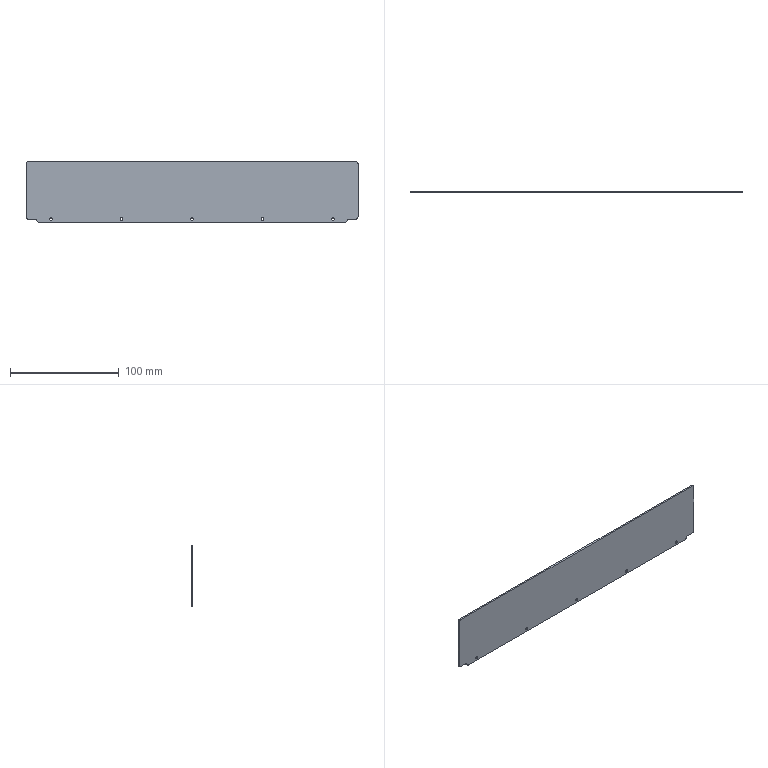Part | NX | features BREP 1 | 1 solid | 36 faces | box 306 x 1.5 x 56 mm | volume 25546 mm3 | cylinder 16 | plane 10 | cone 10 | commonest cylinder face diameters 2.4 x10 4 x6
STEP:
#1=CARTESIAN_POINT('',(-151.,-1.5,28.));
#2=VERTEX_POINT('',#1);
#3=CARTESIAN_POINT('',(-153.,-1.5,26.));
#4=VERTEX_POINT('',#3);
#5=CARTESIAN_POINT('',(-151.,-1.5,26.));
#6=DIRECTION('',(0.,-1.,0.));
#7=DIRECTION('',(0.,0.,1.));
#8=AXIS2_PLACEMENT_3D('',#5,#6,#7);
#9=CIRCLE('',#8,2.);
#10=EDGE_CURVE('',#2,#4,#9,.T.);
#11=ORIENTED_EDGE('',*,*,#10,.F.);
#12=CARTESIAN_POINT('',(-151.,0.,28.));
#13=VERTEX_POINT('',#12);
#14=CARTESIAN_POINT('',(-151.,-1.5,28.));
#15=DIRECTION('',(0.,-1.,0.));
#16=VECTOR('',#15,1000.);
#17=LINE('',#14,#16);
#18=EDGE_CURVE('',#13,#2,#17,.T.);
#19=ORIENTED_EDGE('',*,*,#18,.F.);
#20=CARTESIAN_POINT('',(-153.,0.,26.));
#21=VERTEX_POINT('',#20);
#22=CARTESIAN_POINT('',(-151.,0.,26.));
#23=DIRECTION('',(0.,1.,0.));
#24=DIRECTION('',(0.,0.,1.));
#25=AXIS2_PLACEMENT_3D('',#22,#23,#24);
#26=CIRCLE('',#25,2.);
#27=EDGE_CURVE('',#21,#13,#26,.T.);
#28=ORIENTED_EDGE('',*,*,#27,.F.);
#29=CARTESIAN_POINT('',(-153.,-1.5,26.));
#30=DIRECTION('',(0.,1.,0.));
#31=VECTOR('',#30,1000.);
#32=LINE('',#29,#31);
#33=EDGE_CURVE('',#4,#21,#32,.T.);
#34=ORIENTED_EDGE('',*,*,#33,.F.);
#35=EDGE_LOOP('',(#11,#19,#28,#34));
#36=FACE_BOUND('',#35,.T.);
#37=CARTESIAN_POINT('',(-151.,-1.5,26.));
#38=DIRECTION('',(0.,1.,0.));
#39=DIRECTION('',(0.,0.,1.));
#40=AXIS2_PLACEMENT_3D('',#37,#38,#39);
#41=CYLINDRICAL_SURFACE('',#40,2.);
#42=ADVANCED_FACE('',(#36),#41,.T.);
#43=CARTESIAN_POINT('',(153.,-1.5,26.));
#44=VERTEX_POINT('',#43);
#45=CARTESIAN_POINT('',(151.,-1.5,28.));
#46=VERTEX_POINT('',#45);
#47=CARTESIAN_POINT('',(151.,-1.5,26.));
#48=DIRECTION('',(0.,-1.,0.));
#49=DIRECTION('',(0.,0.,1.));
#50=AXIS2_PLACEMENT_3D('',#47,#48,#49);
#51=CIRCLE('',#50,2.);
#52=EDGE_CURVE('',#44,#46,#51,.T.);
#53=ORIENTED_EDGE('',*,*,#52,.F.);
#54=CARTESIAN_POINT('',(153.,0.,26.));
#55=VERTEX_POINT('',#54);
#56=CARTESIAN_POINT('',(153.,-1.5,26.));
#57=DIRECTION('',(0.,-1.,0.));
#58=VECTOR('',#57,1000.);
#59=LINE('',#56,#58);
#60=EDGE_CURVE('',#55,#44,#59,.T.);
#61=ORIENTED_EDGE('',*,*,#60,.F.);
#62=CARTESIAN_POINT('',(151.,0.,28.));
#63=VERTEX_POINT('',#62);
#64=CARTESIAN_POINT('',(151.,0.,26.));
#65=DIRECTION('',(0.,1.,0.));
#66=DIRECTION('',(0.,0.,1.));
#67=AXIS2_PLACEMENT_3D('',#64,#65,#66);
#68=CIRCLE('',#67,2.);
#69=EDGE_CURVE('',#63,#55,#68,.T.);
#70=ORIENTED_EDGE('',*,*,#69,.F.);
#71=CARTESIAN_POINT('',(151.,-1.5,28.));
#72=DIRECTION('',(0.,1.,0.));
#73=VECTOR('',#72,1000.);
#74=LINE('',#71,#73);
#75=EDGE_CURVE('',#46,#63,#74,.T.);
#76=ORIENTED_EDGE('',*,*,#75,.F.);
#77=EDGE_LOOP('',(#53,#61,#70,#76));
#78=FACE_BOUND('',#77,.T.);
#79=CARTESIAN_POINT('',(151.,-1.5,26.));
#80=DIRECTION('',(0.,1.,0.));
#81=DIRECTION('',(0.,0.,1.));
#82=AXIS2_PLACEMENT_3D('',#79,#80,#81);
#83=CYLINDRICAL_SURFACE('',#82,2.);
#84=ADVANCED_FACE('',(#78),#83,.T.);
#85=CARTESIAN_POINT('',(151.,-1.5,-25.));
#86=VERTEX_POINT('',#85);
#87=CARTESIAN_POINT('',(153.,-1.5,-23.));
#88=VERTEX_POINT('',#87);
#89=CARTESIAN_POINT('',(151.,-1.5,-23.));
#90=DIRECTION('',(0.,-1.,0.));
#91=DIRECTION('',(0.,0.,1.));
#92=AXIS2_PLACEMENT_3D('',#89,#90,#91);
#93=CIRCLE('',#92,2.);
#94=EDGE_CURVE('',#86,#88,#93,.T.);
#95=ORIENTED_EDGE('',*,*,#94,.F.);
#96=CARTESIAN_POINT('',(151.,0.,-25.));
#97=VERTEX_POINT('',#96);
#98=CARTESIAN_POINT('',(151.,-1.5,-25.));
#99=DIRECTION('',(0.,-1.,0.));
#100=VECTOR('',#99,1000.);
#101=LINE('',#98,#100);
#102=EDGE_CURVE('',#97,#86,#101,.T.);
#103=ORIENTED_EDGE('',*,*,#102,.F.);
#104=CARTESIAN_POINT('',(153.,0.,-23.));
#105=VERTEX_POINT('',#104);
#106=CARTESIAN_POINT('',(151.,0.,-23.));
#107=DIRECTION('',(0.,1.,0.));
#108=DIRECTION('',(0.,0.,1.));
#109=AXIS2_PLACEMENT_3D('',#106,#107,#108);
#110=CIRCLE('',#109,2.);
#111=EDGE_CURVE('',#105,#97,#110,.T.);
#112=ORIENTED_EDGE('',*,*,#111,.F.);
#113=CARTESIAN_POINT('',(153.,0.,-23.));
#114=DIRECTION('',(0.,1.,0.));
#115=VECTOR('',#114,1000.);
#116=LINE('',#113,#115);
#117=EDGE_CURVE('',#88,#105,#116,.T.);
#118=ORIENTED_EDGE('',*,*,#117,.F.);
#119=EDGE_LOOP('',(#95,#103,#112,#118));
#120=FACE_BOUND('',#119,.T.);
#121=CARTESIAN_POINT('',(151.,-1.5,-23.));
#122=DIRECTION('',(0.,-1.,0.));
#123=DIRECTION('',(0.,0.,-1.));
#124=AXIS2_PLACEMENT_3D('',#121,#122,#123);
#125=CYLINDRICAL_SURFACE('',#124,2.);
#126=ADVANCED_FACE('',(#120),#125,.T.);
#127=CARTESIAN_POINT('',(-153.,-1.5,-23.));
#128=VERTEX_POINT('',#127);
#129=CARTESIAN_POINT('',(-151.,-1.5,-25.));
#130=VERTEX_POINT('',#129);
#131=CARTESIAN_POINT('',(-151.,-1.5,-23.));
#132=DIRECTION('',(0.,-1.,0.));
#133=DIRECTION('',(0.,0.,1.));
#134=AXIS2_PLACEMENT_3D('',#131,#132,#133);
#135=CIRCLE('',#134,2.);
#136=EDGE_CURVE('',#128,#130,#135,.T.);
#137=ORIENTED_EDGE('',*,*,#136,.F.);
#138=CARTESIAN_POINT('',(-153.,0.,-23.));
#139=VERTEX_POINT('',#138);
#140=CARTESIAN_POINT('',(-153.,-1.5,-23.));
#141=DIRECTION('',(0.,-1.,0.));
#142=VECTOR('',#141,1000.);
#143=LINE('',#140,#142);
#144=EDGE_CURVE('',#139,#128,#143,.T.);
#145=ORIENTED_EDGE('',*,*,#144,.F.);
#146=CARTESIAN_POINT('',(-151.,0.,-25.));
#147=VERTEX_POINT('',#146);
#148=CARTESIAN_POINT('',(-151.,0.,-23.));
#149=DIRECTION('',(0.,1.,0.));
#150=DIRECTION('',(0.,0.,1.));
#151=AXIS2_PLACEMENT_3D('',#148,#149,#150);
#152=CIRCLE('',#151,2.);
#153=EDGE_CURVE('',#147,#139,#152,.T.);
#154=ORIENTED_EDGE('',*,*,#153,.F.);
#155=CARTESIAN_POINT('',(-151.,0.,-25.));
#156=DIRECTION('',(0.,1.,0.));
#157=VECTOR('',#156,1000.);
#158=LINE('',#155,#157);
#159=EDGE_CURVE('',#130,#147,#158,.T.);
#160=ORIENTED_EDGE('',*,*,#159,.F.);
#161=EDGE_LOOP('',(#137,#145,#154,#160));
#162=FACE_BOUND('',#161,.T.);
#163=CARTESIAN_POINT('',(-151.,-1.5,-23.));
#164=DIRECTION('',(0.,-1.,0.));
#165=DIRECTION('',(0.,0.,-1.));
#166=AXIS2_PLACEMENT_3D('',#163,#164,#165);
#167=CYLINDRICAL_SURFACE('',#166,2.);
#168=ADVANCED_FACE('',(#162),#167,.T.);
#169=CARTESIAN_POINT('',(-143.,-1.5,-26.));
#170=VERTEX_POINT('',#169);
#171=CARTESIAN_POINT('',(-141.,-1.5,-28.));
#172=VERTEX_POINT('',#171);
#173=CARTESIAN_POINT('',(-141.,-1.5,-26.));
#174=DIRECTION('',(0.,-1.,0.));
#175=DIRECTION('',(0.,0.,1.));
#176=AXIS2_PLACEMENT_3D('',#173,#174,#175);
#177=CIRCLE('',#176,2.);
#178=EDGE_CURVE('',#170,#172,#177,.T.);
#179=ORIENTED_EDGE('',*,*,#178,.F.);
#180=CARTESIAN_POINT('',(-143.,0.,-26.));
#181=VERTEX_POINT('',#180);
#182=CARTESIAN_POINT('',(-143.,-1.5,-26.));
#183=DIRECTION('',(0.,-1.,0.));
#184=VECTOR('',#183,1000.);
#185=LINE('',#182,#184);
#186=EDGE_CURVE('',#181,#170,#185,.T.);
#187=ORIENTED_EDGE('',*,*,#186,.F.);
#188=CARTESIAN_POINT('',(-141.,0.,-28.));
#189=VERTEX_POINT('',#188);
#190=CARTESIAN_POINT('',(-141.,0.,-26.));
#191=DIRECTION('',(0.,1.,0.));
#192=DIRECTION('',(0.,0.,1.));
#193=AXIS2_PLACEMENT_3D('',#190,#191,#192);
#194=CIRCLE('',#193,2.);
#195=EDGE_CURVE('',#189,#181,#194,.T.);
#196=ORIENTED_EDGE('',*,*,#195,.F.);
#197=CARTESIAN_POINT('',(-141.,0.,-28.));
#198=DIRECTION('',(0.,1.,0.));
#199=VECTOR('',#198,1000.);
#200=LINE('',#197,#199);
#201=EDGE_CURVE('',#172,#189,#200,.T.);
#202=ORIENTED_EDGE('',*,*,#201,.F.);
#203=EDGE_LOOP('',(#179,#187,#196,#202));
#204=FACE_BOUND('',#203,.T.);
#205=CARTESIAN_POINT('',(-141.,-1.5,-26.));
#206=DIRECTION('',(0.,-1.,0.));
#207=DIRECTION('',(0.,0.,-1.));
#208=AXIS2_PLACEMENT_3D('',#205,#206,#207);
#209=CYLINDRICAL_SURFACE('',#208,2.);
#210=ADVANCED_FACE('',(#204),#209,.T.);
#211=CARTESIAN_POINT('',(141.,-1.5,-28.));
#212=VERTEX_POINT('',#211);
#213=CARTESIAN_POINT('',(143.,-1.5,-26.));
#214=VERTEX_POINT('',#213);
#215=CARTESIAN_POINT('',(141.,-1.5,-26.));
#216=DIRECTION('',(0.,-1.,0.));
#217=DIRECTION('',(0.,0.,1.));
#218=AXIS2_PLACEMENT_3D('',#215,#216,#217);
#219=CIRCLE('',#218,2.);
#220=EDGE_CURVE('',#212,#214,#219,.T.);
#221=ORIENTED_EDGE('',*,*,#220,.F.);
#222=CARTESIAN_POINT('',(141.,0.,-28.));
#223=VERTEX_POINT('',#222);
#224=CARTESIAN_POINT('',(141.,-1.5,-28.));
#225=DIRECTION('',(0.,-1.,0.));
#226=VECTOR('',#225,1000.);
#227=LINE('',#224,#226);
#228=EDGE_CURVE('',#223,#212,#227,.T.);
#229=ORIENTED_EDGE('',*,*,#228,.F.);
#230=CARTESIAN_POINT('',(143.,0.,-26.));
#231=VERTEX_POINT('',#230);
#232=CARTESIAN_POINT('',(141.,0.,-26.));
#233=DIRECTION('',(0.,1.,0.));
#234=DIRECTION('',(0.,0.,1.));
#235=AXIS2_PLACEMENT_3D('',#232,#233,#234);
#236=CIRCLE('',#235,2.);
#237=EDGE_CURVE('',#231,#223,#236,.T.);
#238=ORIENTED_EDGE('',*,*,#237,.F.);
#239=CARTESIAN_POINT('',(143.,0.,-26.));
#240=DIRECTION('',(0.,1.,0.));
#241=VECTOR('',#240,1000.);
#242=LINE('',#239,#241);
#243=EDGE_CURVE('',#214,#231,#242,.T.);
#244=ORIENTED_EDGE('',*,*,#243,.F.);
#245=EDGE_LOOP('',(#221,#229,#238,#244));
#246=FACE_BOUND('',#245,.T.);
#247=CARTESIAN_POINT('',(141.,-1.5,-26.));
#248=DIRECTION('',(0.,-1.,0.));
#249=DIRECTION('',(0.,0.,-1.));
#250=AXIS2_PLACEMENT_3D('',#247,#248,#249);
#251=CYLINDRICAL_SURFACE('',#250,2.);
#252=ADVANCED_FACE('',(#246),#251,.T.);
#253=CARTESIAN_POINT('',(-143.,-1.5,-25.));
#254=VERTEX_POINT('',#253);
#255=CARTESIAN_POINT('',(-153.,-1.5,-25.));
#256=DIRECTION('',(1.,0.,0.));
#257=VECTOR('',#256,1000.);
#258=LINE('',#255,#257);
#259=EDGE_CURVE('',#130,#254,#258,.T.);
#260=ORIENTED_EDGE('',*,*,#259,.F.);
#261=ORIENTED_EDGE('',*,*,#159,.T.);
#262=CARTESIAN_POINT('',(-143.,0.,-25.));
#263=VERTEX_POINT('',#262);
#264=CARTESIAN_POINT('',(-153.,0.,-25.));
#265=DIRECTION('',(1.,0.,0.));
#266=VECTOR('',#265,1000.);
#267=LINE('',#264,#266);
#268=EDGE_CURVE('',#147,#263,#267,.T.);
#269=ORIENTED_EDGE('',*,*,#268,.T.);
#270=CARTESIAN_POINT('',(-143.,-1.5,-25.));
#271=DIRECTION('',(0.,1.,0.));
#272=VECTOR('',#271,1000.);
#273=LINE('',#270,#272);
#274=EDGE_CURVE('',#254,#263,#273,.T.);
#275=ORIENTED_EDGE('',*,*,#274,.F.);
#276=EDGE_LOOP('',(#260,#261,#269,#275));
#277=FACE_BOUND('',#276,.T.);
#278=CARTESIAN_POINT('',(-153.,-1.5,-25.));
#279=DIRECTION('',(0.,0.,1.));
#280=DIRECTION('',(1.,0.,0.));
#281=AXIS2_PLACEMENT_3D('',#278,#279,#280);
#282=PLANE('',#281);
#283=ADVANCED_FACE('',(#277),#282,.F.);
#284=CARTESIAN_POINT('',(-143.,0.,-28.));
#285=DIRECTION('',(0.,0.,-1.));
#286=VECTOR('',#285,1000.);
#287=LINE('',#284,#286);
#288=EDGE_CURVE('',#263,#181,#287,.T.);
#289=ORIENTED_EDGE('',*,*,#288,.T.);
#290=ORIENTED_EDGE('',*,*,#186,.T.);
#291=CARTESIAN_POINT('',(-143.,-1.5,-28.));
#292=DIRECTION('',(0.,0.,-1.));
#293=VECTOR('',#292,1000.);
#294=LINE('',#291,#293);
#295=EDGE_CURVE('',#254,#170,#294,.T.);
#296=ORIENTED_EDGE('',*,*,#295,.F.);
#297=ORIENTED_EDGE('',*,*,#274,.T.);
#298=EDGE_LOOP('',(#289,#290,#296,#297));
#299=FACE_BOUND('',#298,.T.);
#300=CARTESIAN_POINT('',(-143.,-1.5,-28.));
#301=DIRECTION('',(1.,0.,0.));
#302=DIRECTION('',(0.,0.,-1.));
#303=AXIS2_PLACEMENT_3D('',#300,#301,#302);
#304=PLANE('',#303);
#305=ADVANCED_FACE('',(#299),#304,.F.);
#306=CARTESIAN_POINT('',(143.,-1.5,-25.));
#307=VERTEX_POINT('',#306);
#308=CARTESIAN_POINT('',(143.,-1.5,-28.));
#309=DIRECTION('',(0.,0.,1.));
#310=VECTOR('',#309,1000.);
#311=LINE('',#308,#310);
#312=EDGE_CURVE('',#214,#307,#311,.T.);
#313=ORIENTED_EDGE('',*,*,#312,.F.);
#314=ORIENTED_EDGE('',*,*,#243,.T.);
#315=CARTESIAN_POINT('',(143.,0.,-25.));
#316=VERTEX_POINT('',#315);
#317=CARTESIAN_POINT('',(143.,0.,-28.));
#318=DIRECTION('',(0.,0.,1.));
#319=VECTOR('',#318,1000.);
#320=LINE('',#317,#319);
#321=EDGE_CURVE('',#231,#316,#320,.T.);
#322=ORIENTED_EDGE('',*,*,#321,.T.);
#323=CARTESIAN_POINT('',(143.,-1.5,-25.));
#324=DIRECTION('',(0.,1.,0.));
#325=VECTOR('',#324,1000.);
#326=LINE('',#323,#325);
#327=EDGE_CURVE('',#307,#316,#326,.T.);
#328=ORIENTED_EDGE('',*,*,#327,.F.);
#329=EDGE_LOOP('',(#313,#314,#322,#328));
#330=FACE_BOUND('',#329,.T.);
#331=CARTESIAN_POINT('',(143.,-1.5,-28.));
#332=DIRECTION('',(-1.,0.,0.));
#333=DIRECTION('',(0.,0.,1.));
#334=AXIS2_PLACEMENT_3D('',#331,#332,#333);
#335=PLANE('',#334);
#336=ADVANCED_FACE('',(#330),#335,.F.);
#337=CARTESIAN_POINT('',(153.,0.,-25.));
#338=DIRECTION('',(1.,0.,0.));
#339=VECTOR('',#338,1000.);
#340=LINE('',#337,#339);
#341=EDGE_CURVE('',#316,#97,#340,.T.);
#342=ORIENTED_EDGE('',*,*,#341,.T.);
#343=ORIENTED_EDGE('',*,*,#102,.T.);
#344=CARTESIAN_POINT('',(153.,-1.5,-25.));
#345=DIRECTION('',(1.,0.,0.));
#346=VECTOR('',#345,1000.);
#347=LINE('',#344,#346);
#348=EDGE_CURVE('',#307,#86,#347,.T.);
#349=ORIENTED_EDGE('',*,*,#348,.F.);
#350=ORIENTED_EDGE('',*,*,#327,.T.);
#351=EDGE_LOOP('',(#342,#343,#349,#350));
#352=FACE_BOUND('',#351,.T.);
#353=CARTESIAN_POINT('',(153.,-1.5,-25.));
#354=DIRECTION('',(0.,0.,1.));
#355=DIRECTION('',(1.,0.,0.));
#356=AXIS2_PLACEMENT_3D('',#353,#354,#355);
#357=PLANE('',#356);
#358=ADVANCED_FACE('',(#352),#357,.F.);
#359=CARTESIAN_POINT('',(-130.,0.,-27.25));
#360=VERTEX_POINT('',#359);
#361=CARTESIAN_POINT('',(-130.,-1.05,-26.2));
#362=VERTEX_POINT('',#361);
#363=CARTESIAN_POINT('',(-130.,0.,-27.25));
#364=DIRECTION('',(0.,0.7071,-0.7071));
#365=VECTOR('',#364,1000.);
#366=LINE('',#363,#365);
#367=EDGE_CURVE('',#360,#362,#366,.F.);
#368=ORIENTED_EDGE('',*,*,#367,.T.);
#369=CARTESIAN_POINT('',(-130.,-1.05,-23.8));
#370=VERTEX_POINT('',#369);
#371=CARTESIAN_POINT('',(-130.,-1.05,-25.));
#372=DIRECTION('',(0.,1.,0.));
#373=DIRECTION('',(0.,0.,1.));
#374=AXIS2_PLACEMENT_3D('',#371,#372,#373);
#375=CIRCLE('',#374,1.2);
#376=EDGE_CURVE('',#370,#362,#375,.T.);
#377=ORIENTED_EDGE('',*,*,#376,.F.);
#378=CARTESIAN_POINT('',(-130.,0.,-22.75));
#379=VERTEX_POINT('',#378);
#380=CARTESIAN_POINT('',(-130.,0.,-22.75));
#381=DIRECTION('',(0.,0.7071,0.7071));
#382=VECTOR('',#381,1000.);
#383=LINE('',#380,#382);
#384=EDGE_CURVE('',#379,#370,#383,.F.);
#385=ORIENTED_EDGE('',*,*,#384,.F.);
#386=CARTESIAN_POINT('',(-130.,0.,-25.));
#387=DIRECTION('',(0.,1.,0.));
#388=DIRECTION('',(0.,0.,1.));
#389=AXIS2_PLACEMENT_3D('',#386,#387,#388);
#390=CIRCLE('',#389,2.25);
#391=EDGE_CURVE('',#379,#360,#390,.T.);
#392=ORIENTED_EDGE('',*,*,#391,.T.);
#393=EDGE_LOOP('',(#368,#377,#385,#392));
#394=FACE_BOUND('',#393,.T.);
#395=CARTESIAN_POINT('',(-130.,0.,-25.));
#396=DIRECTION('',(0.,1.,0.));
#397=DIRECTION('',(0.,0.,1.));
#398=AXIS2_PLACEMENT_3D('',#395,#396,#397);
#399=CONICAL_SURFACE('',#398,2.25,0.7854);
#400=ADVANCED_FACE('',(#394),#399,.F.);
#401=CARTESIAN_POINT('',(-130.,-1.5,-26.2));
#402=VERTEX_POINT('',#401);
#403=CARTESIAN_POINT('',(-130.,0.,-26.2));
#404=DIRECTION('',(0.,1.,0.));
#405=VECTOR('',#404,1000.);
#406=LINE('',#403,#405);
#407=EDGE_CURVE('',#362,#402,#406,.F.);
#408=ORIENTED_EDGE('',*,*,#407,.T.);
#409=CARTESIAN_POINT('',(-130.,-1.5,-23.8));
#410=VERTEX_POINT('',#409);
#411=CARTESIAN_POINT('',(-130.,-1.5,-25.));
#412=DIRECTION('',(0.,1.,0.));
#413=DIRECTION('',(0.,0.,1.));
#414=AXIS2_PLACEMENT_3D('',#411,#412,#413);
#415=CIRCLE('',#414,1.2);
#416=EDGE_CURVE('',#410,#402,#415,.T.);
#417=ORIENTED_EDGE('',*,*,#416,.F.);
#418=CARTESIAN_POINT('',(-130.,0.,-23.8));
#419=DIRECTION('',(0.,1.,0.));
#420=VECTOR('',#419,1000.);
#421=LINE('',#418,#420);
#422=EDGE_CURVE('',#370,#410,#421,.F.);
#423=ORIENTED_EDGE('',*,*,#422,.F.);
#424=ORIENTED_EDGE('',*,*,#376,.T.);
#425=EDGE_LOOP('',(#408,#417,#423,#424));
#426=FACE_BOUND('',#425,.T.);
#427=CARTESIAN_POINT('',(-130.,0.,-25.));
#428=DIRECTION('',(0.,1.,0.));
#429=DIRECTION('',(0.,0.,1.));
#430=AXIS2_PLACEMENT_3D('',#427,#428,#429);
#431=CYLINDRICAL_SURFACE('',#430,1.2);
#432=ADVANCED_FACE('',(#426),#431,.F.);
#433=CARTESIAN_POINT('',(-65.,0.,-27.25));
#434=VERTEX_POINT('',#433);
#435=CARTESIAN_POINT('',(-65.,-1.05,-26.2));
#436=VERTEX_POINT('',#435);
#437=CARTESIAN_POINT('',(-65.,0.,-27.25));
#438=DIRECTION('',(0.,0.7071,-0.7071));
#439=VECTOR('',#438,1000.);
#440=LINE('',#437,#439);
#441=EDGE_CURVE('',#434,#436,#440,.F.);
#442=ORIENTED_EDGE('',*,*,#441,.T.);
#443=CARTESIAN_POINT('',(-65.,-1.05,-23.8));
#444=VERTEX_POINT('',#443);
#445=CARTESIAN_POINT('',(-65.,-1.05,-25.));
#446=DIRECTION('',(0.,1.,0.));
#447=DIRECTION('',(0.,0.,1.));
#448=AXIS2_PLACEMENT_3D('',#445,#446,#447);
#449=CIRCLE('',#448,1.2);
#450=EDGE_CURVE('',#444,#436,#449,.T.);
#451=ORIENTED_EDGE('',*,*,#450,.F.);
#452=CARTESIAN_POINT('',(-65.,0.,-22.75));
#453=VERTEX_POINT('',#452);
#454=CARTESIAN_POINT('',(-65.,0.,-22.75));
#455=DIRECTION('',(0.,0.7071,0.7071));
#456=VECTOR('',#455,1000.);
#457=LINE('',#454,#456);
#458=EDGE_CURVE('',#453,#444,#457,.F.);
#459=ORIENTED_EDGE('',*,*,#458,.F.);
#460=CARTESIAN_POINT('',(-65.,0.,-25.));
#461=DIRECTION('',(0.,1.,0.));
#462=DIRECTION('',(0.,0.,1.));
#463=AXIS2_PLACEMENT_3D('',#460,#461,#462);
#464=CIRCLE('',#463,2.25);
#465=EDGE_CURVE('',#453,#434,#464,.T.);
#466=ORIENTED_EDGE('',*,*,#465,.T.);
#467=EDGE_LOOP('',(#442,#451,#459,#466));
#468=FACE_BOUND('',#467,.T.);
#469=CARTESIAN_POINT('',(-65.,0.,-25.));
#470=DIRECTION('',(0.,1.,0.));
#471=DIRECTION('',(0.,0.,1.));
#472=AXIS2_PLACEMENT_3D('',#469,#470,#471);
#473=CONICAL_SURFACE('',#472,2.25,0.7854);
#474=ADVANCED_FACE('',(#468),#473,.F.);
#475=CARTESIAN_POINT('',(-65.,-1.5,-26.2));
#476=VERTEX_POINT('',#475);
#477=CARTESIAN_POINT('',(-65.,0.,-26.2));
#478=DIRECTION('',(0.,1.,0.));
#479=VECTOR('',#478,1000.);
#480=LINE('',#477,#479);
#481=EDGE_CURVE('',#436,#476,#480,.F.);
#482=ORIENTED_EDGE('',*,*,#481,.T.);
#483=CARTESIAN_POINT('',(-65.,-1.5,-23.8));
#484=VERTEX_POINT('',#483);
#485=CARTESIAN_POINT('',(-65.,-1.5,-25.));
#486=DIRECTION('',(0.,1.,0.));
#487=DIRECTION('',(0.,0.,1.));
#488=AXIS2_PLACEMENT_3D('',#485,#486,#487);
#489=CIRCLE('',#488,1.2);
#490=EDGE_CURVE('',#484,#476,#489,.T.);
#491=ORIENTED_EDGE('',*,*,#490,.F.);
#492=CARTESIAN_POINT('',(-65.,0.,-23.8));
#493=DIRECTION('',(0.,1.,0.));
#494=VECTOR('',#493,1000.);
#495=LINE('',#492,#494);
#496=EDGE_CURVE('',#444,#484,#495,.F.);
#497=ORIENTED_EDGE('',*,*,#496,.F.);
#498=ORIENTED_EDGE('',*,*,#450,.T.);
#499=EDGE_LOOP('',(#482,#491,#497,#498));
#500=FACE_BOUND('',#499,.T.);
#501=CARTESIAN_POINT('',(-65.,0.,-25.));
#502=DIRECTION('',(0.,1.,0.));
#503=DIRECTION('',(0.,0.,1.));
#504=AXIS2_PLACEMENT_3D('',#501,#502,#503);
#505=CYLINDRICAL_SURFACE('',#504,1.2);
#506=ADVANCED_FACE('',(#500),#505,.F.);
#507=CARTESIAN_POINT('',(0.,0.,-27.25));
#508=VERTEX_POINT('',#507);
#509=CARTESIAN_POINT('',(0.,-1.05,-26.2));
#510=VERTEX_POINT('',#509);
#511=CARTESIAN_POINT('',(0.,0.,-27.25));
#512=DIRECTION('',(0.,0.7071,-0.7071));
#513=VECTOR('',#512,1000.);
#514=LINE('',#511,#513);
#515=EDGE_CURVE('',#508,#510,#514,.F.);
#516=ORIENTED_EDGE('',*,*,#515,.T.);
#517=CARTESIAN_POINT('',(0.,-1.05,-23.8));
#518=VERTEX_POINT('',#517);
#519=CARTESIAN_POINT('',(0.,-1.05,-25.));
#520=DIRECTION('',(0.,1.,0.));
#521=DIRECTION('',(0.,0.,1.));
#522=AXIS2_PLACEMENT_3D('',#519,#520,#521);
#523=CIRCLE('',#522,1.2);
#524=EDGE_CURVE('',#518,#510,#523,.T.);
#525=ORIENTED_EDGE('',*,*,#524,.F.);
#526=CARTESIAN_POINT('',(0.,0.,-22.75));
#527=VERTEX_POINT('',#526);
#528=CARTESIAN_POINT('',(0.,0.,-22.75));
#529=DIRECTION('',(0.,0.7071,0.7071));
#530=VECTOR('',#529,1000.);
#531=LINE('',#528,#530);
#532=EDGE_CURVE('',#527,#518,#531,.F.);
#533=ORIENTED_EDGE('',*,*,#532,.F.);
#534=CARTESIAN_POINT('',(0.,0.,-25.));
#535=DIRECTION('',(0.,1.,0.));
#536=DIRECTION('',(0.,0.,1.));
#537=AXIS2_PLACEMENT_3D('',#534,#535,#536);
#538=CIRCLE('',#537,2.25);
#539=EDGE_CURVE('',#527,#508,#538,.T.);
#540=ORIENTED_EDGE('',*,*,#539,.T.);
#541=EDGE_LOOP('',(#516,#525,#533,#540));
#542=FACE_BOUND('',#541,.T.);
#543=CARTESIAN_POINT('',(0.,0.,-25.));
#544=DIRECTION('',(0.,1.,0.));
#545=DIRECTION('',(0.,0.,1.));
#546=AXIS2_PLACEMENT_3D('',#543,#544,#545);
#547=CONICAL_SURFACE('',#546,2.25,0.7854);
#548=ADVANCED_FACE('',(#542),#547,.F.);
#549=CARTESIAN_POINT('',(0.,-1.5,-26.2));
#550=VERTEX_POINT('',#549);
#551=CARTESIAN_POINT('',(0.,0.,-26.2));
#552=DIRECTION('',(0.,1.,0.));
#553=VECTOR('',#552,1000.);
#554=LINE('',#551,#553);
#555=EDGE_CURVE('',#510,#550,#554,.F.);
#556=ORIENTED_EDGE('',*,*,#555,.T.);
#557=CARTESIAN_POINT('',(0.,-1.5,-23.8));
#558=VERTEX_POINT('',#557);
#559=CARTESIAN_POINT('',(0.,-1.5,-25.));
#560=DIRECTION('',(0.,1.,0.));
#561=DIRECTION('',(0.,0.,1.));
#562=AXIS2_PLACEMENT_3D('',#559,#560,#561);
#563=CIRCLE('',#562,1.2);
#564=EDGE_CURVE('',#558,#550,#563,.T.);
#565=ORIENTED_EDGE('',*,*,#564,.F.);
#566=CARTESIAN_POINT('',(0.,0.,-23.8));
#567=DIRECTION('',(0.,1.,0.));
#568=VECTOR('',#567,1000.);
#569=LINE('',#566,#568);
#570=EDGE_CURVE('',#518,#558,#569,.F.);
#571=ORIENTED_EDGE('',*,*,#570,.F.);
#572=ORIENTED_EDGE('',*,*,#524,.T.);
#573=EDGE_LOOP('',(#556,#565,#571,#572));
#574=FACE_BOUND('',#573,.T.);
#575=CARTESIAN_POINT('',(0.,0.,-25.));
#576=DIRECTION('',(0.,1.,0.));
#577=DIRECTION('',(0.,0.,1.));
#578=AXIS2_PLACEMENT_3D('',#575,#576,#577);
#579=CYLINDRICAL_SURFACE('',#578,1.2);
#580=ADVANCED_FACE('',(#574),#579,.F.);
#581=CARTESIAN_POINT('',(65.,0.,-27.25));
#582=VERTEX_POINT('',#581);
#583=CARTESIAN_POINT('',(65.,-1.05,-26.2));
#584=VERTEX_POINT('',#583);
#585=CARTESIAN_POINT('',(65.,0.,-27.25));
#586=DIRECTION('',(0.,0.7071,-0.7071));
#587=VECTOR('',#586,1000.);
#588=LINE('',#585,#587);
#589=EDGE_CURVE('',#582,#584,#588,.F.);
#590=ORIENTED_EDGE('',*,*,#589,.T.);
#591=CARTESIAN_POINT('',(65.,-1.05,-23.8));
#592=VERTEX_POINT('',#591);
#593=CARTESIAN_POINT('',(65.,-1.05,-25.));
#594=DIRECTION('',(0.,1.,0.));
#595=DIRECTION('',(0.,0.,1.));
#596=AXIS2_PLACEMENT_3D('',#593,#594,#595);
#597=CIRCLE('',#596,1.2);
#598=EDGE_CURVE('',#592,#584,#597,.T.);
#599=ORIENTED_EDGE('',*,*,#598,.F.);
#600=CARTESIAN_POINT('',(65.,0.,-22.75));
#601=VERTEX_POINT('',#600);
#602=CARTESIAN_POINT('',(65.,0.,-22.75));
#603=DIRECTION('',(0.,0.7071,0.7071));
#604=VECTOR('',#603,1000.);
#605=LINE('',#602,#604);
#606=EDGE_CURVE('',#601,#592,#605,.F.);
#607=ORIENTED_EDGE('',*,*,#606,.F.);
#608=CARTESIAN_POINT('',(65.,0.,-25.));
#609=DIRECTION('',(0.,1.,0.));
#610=DIRECTION('',(0.,0.,1.));
#611=AXIS2_PLACEMENT_3D('',#608,#609,#610);
#612=CIRCLE('',#611,2.25);
#613=EDGE_CURVE('',#601,#582,#612,.T.);
#614=ORIENTED_EDGE('',*,*,#613,.T.);
#615=EDGE_LOOP('',(#590,#599,#607,#614));
#616=FACE_BOUND('',#615,.T.);
#617=CARTESIAN_POINT('',(65.,0.,-25.));
#618=DIRECTION('',(0.,1.,0.));
#619=DIRECTION('',(0.,0.,1.));
#620=AXIS2_PLACEMENT_3D('',#617,#618,#619);
#621=CONICAL_SURFACE('',#620,2.25,0.7854);
#622=ADVANCED_FACE('',(#616),#621,.F.);
#623=CARTESIAN_POINT('',(65.,-1.5,-26.2));
#624=VERTEX_POINT('',#623);
#625=CARTESIAN_POINT('',(65.,0.,-26.2));
#626=DIRECTION('',(0.,1.,0.));
#627=VECTOR('',#626,1000.);
#628=LINE('',#625,#627);
#629=EDGE_CURVE('',#584,#624,#628,.F.);
#630=ORIENTED_EDGE('',*,*,#629,.T.);
#631=CARTESIAN_POINT('',(65.,-1.5,-23.8));
#632=VERTEX_POINT('',#631);
#633=CARTESIAN_POINT('',(65.,-1.5,-25.));
#634=DIRECTION('',(0.,1.,0.));
#635=DIRECTION('',(0.,0.,1.));
#636=AXIS2_PLACEMENT_3D('',#633,#634,#635);
#637=CIRCLE('',#636,1.2);
#638=EDGE_CURVE('',#632,#624,#637,.T.);
#639=ORIENTED_EDGE('',*,*,#638,.F.);
#640=CARTESIAN_POINT('',(65.,0.,-23.8));
#641=DIRECTION('',(0.,1.,0.));
#642=VECTOR('',#641,1000.);
#643=LINE('',#640,#642);
#644=EDGE_CURVE('',#592,#632,#643,.F.);
#645=ORIENTED_EDGE('',*,*,#644,.F.);
#646=ORIENTED_EDGE('',*,*,#598,.T.);
#647=EDGE_LOOP('',(#630,#639,#645,#646));
#648=FACE_BOUND('',#647,.T.);
#649=CARTESIAN_POINT('',(65.,0.,-25.));
#650=DIRECTION('',(0.,1.,0.));
#651=DIRECTION('',(0.,0.,1.));
#652=AXIS2_PLACEMENT_3D('',#649,#650,#651);
#653=CYLINDRICAL_SURFACE('',#652,1.2);
#654=ADVANCED_FACE('',(#648),#653,.F.);
#655=CARTESIAN_POINT('',(130.,0.,-27.25));
#656=VERTEX_POINT('',#655);
#657=CARTESIAN_POINT('',(130.,-1.05,-26.2));
#658=VERTEX_POINT('',#657);
#659=CARTESIAN_POINT('',(130.,0.,-27.25));
#660=DIRECTION('',(0.,0.7071,-0.7071));
#661=VECTOR('',#660,1000.);
#662=LINE('',#659,#661);
#663=EDGE_CURVE('',#656,#658,#662,.F.);
#664=ORIENTED_EDGE('',*,*,#663,.T.);
#665=CARTESIAN_POINT('',(130.,-1.05,-23.8));
#666=VERTEX_POINT('',#665);
#667=CARTESIAN_POINT('',(130.,-1.05,-25.));
#668=DIRECTION('',(0.,1.,0.));
#669=DIRECTION('',(0.,0.,1.));
#670=AXIS2_PLACEMENT_3D('',#667,#668,#669);
#671=CIRCLE('',#670,1.2);
#672=EDGE_CURVE('',#666,#658,#671,.T.);
#673=ORIENTED_EDGE('',*,*,#672,.F.);
#674=CARTESIAN_POINT('',(130.,0.,-22.75));
#675=VERTEX_POINT('',#674);
#676=CARTESIAN_POINT('',(130.,0.,-22.75));
#677=DIRECTION('',(0.,0.7071,0.7071));
#678=VECTOR('',#677,1000.);
#679=LINE('',#676,#678);
#680=EDGE_CURVE('',#675,#666,#679,.F.);
#681=ORIENTED_EDGE('',*,*,#680,.F.);
#682=CARTESIAN_POINT('',(130.,0.,-25.));
#683=DIRECTION('',(0.,1.,0.));
#684=DIRECTION('',(0.,0.,1.));
#685=AXIS2_PLACEMENT_3D('',#682,#683,#684);
#686=CIRCLE('',#685,2.25);
#687=EDGE_CURVE('',#675,#656,#686,.T.);
#688=ORIENTED_EDGE('',*,*,#687,.T.);
#689=EDGE_LOOP('',(#664,#673,#681,#688));
#690=FACE_BOUND('',#689,.T.);
#691=CARTESIAN_POINT('',(130.,0.,-25.));
#692=DIRECTION('',(0.,1.,0.));
#693=DIRECTION('',(0.,0.,1.));
#694=AXIS2_PLACEMENT_3D('',#691,#692,#693);
#695=CONICAL_SURFACE('',#694,2.25,0.7854);
#696=ADVANCED_FACE('',(#690),#695,.F.);
#697=CARTESIAN_POINT('',(130.,-1.5,-26.2));
#698=VERTEX_POINT('',#697);
#699=CARTESIAN_POINT('',(130.,0.,-26.2));
#700=DIRECTION('',(0.,1.,0.));
#701=VECTOR('',#700,1000.);
#702=LINE('',#699,#701);
#703=EDGE_CURVE('',#658,#698,#702,.F.);
#704=ORIENTED_EDGE('',*,*,#703,.T.);
#705=CARTESIAN_POINT('',(130.,-1.5,-23.8));
#706=VERTEX_POINT('',#705);
#707=CARTESIAN_POINT('',(130.,-1.5,-25.));
#708=DIRECTION('',(0.,1.,0.));
#709=DIRECTION('',(0.,0.,1.));
#710=AXIS2_PLACEMENT_3D('',#707,#708,#709);
#711=CIRCLE('',#710,1.2);
#712=EDGE_CURVE('',#706,#698,#711,.T.);
#713=ORIENTED_EDGE('',*,*,#712,.F.);
#714=CARTESIAN_POINT('',(130.,0.,-23.8));
#715=DIRECTION('',(0.,1.,0.));
#716=VECTOR('',#715,1000.);
#717=LINE('',#714,#716);
#718=EDGE_CURVE('',#666,#706,#717,.F.);
#719=ORIENTED_EDGE('',*,*,#718,.F.);
#720=ORIENTED_EDGE('',*,*,#672,.T.);
#721=EDGE_LOOP('',(#704,#713,#719,#720));
#722=FACE_BOUND('',#721,.T.);
#723=CARTESIAN_POINT('',(130.,0.,-25.));
#724=DIRECTION('',(0.,1.,0.));
#725=DIRECTION('',(0.,0.,1.));
#726=AXIS2_PLACEMENT_3D('',#723,#724,#725);
#727=CYLINDRICAL_SURFACE('',#726,1.2);
#728=ADVANCED_FACE('',(#722),#727,.F.);
#729=ORIENTED_EDGE('',*,*,#687,.F.);
#730=CARTESIAN_POINT('',(130.,0.,-25.));
#731=DIRECTION('',(0.,1.,0.));
#732=DIRECTION('',(0.,0.,1.));
#733=AXIS2_PLACEMENT_3D('',#730,#731,#732);
#734=CIRCLE('',#733,2.25);
#735=EDGE_CURVE('',#656,#675,#734,.T.);
#736=ORIENTED_EDGE('',*,*,#735,.F.);
#737=EDGE_LOOP('',(#729,#736));
#738=FACE_BOUND('',#737,.T.);
#739=ORIENTED_EDGE('',*,*,#613,.F.);
#740=CARTESIAN_POINT('',(65.,0.,-25.));
#741=DIRECTION('',(0.,1.,0.));
#742=DIRECTION('',(0.,0.,1.));
#743=AXIS2_PLACEMENT_3D('',#740,#741,#742);
#744=CIRCLE('',#743,2.25);
#745=EDGE_CURVE('',#582,#601,#744,.T.);
#746=ORIENTED_EDGE('',*,*,#745,.F.);
#747=EDGE_LOOP('',(#739,#746));
#748=FACE_BOUND('',#747,.T.);
#749=ORIENTED_EDGE('',*,*,#539,.F.);
#750=CARTESIAN_POINT('',(0.,0.,-25.));
#751=DIRECTION('',(0.,1.,0.));
#752=DIRECTION('',(0.,0.,1.));
#753=AXIS2_PLACEMENT_3D('',#750,#751,#752);
#754=CIRCLE('',#753,2.25);
#755=EDGE_CURVE('',#508,#527,#754,.T.);
#756=ORIENTED_EDGE('',*,*,#755,.F.);
#757=EDGE_LOOP('',(#749,#756));
#758=FACE_BOUND('',#757,.T.);
#759=ORIENTED_EDGE('',*,*,#465,.F.);
#760=CARTESIAN_POINT('',(-65.,0.,-25.));
#761=DIRECTION('',(0.,1.,0.));
#762=DIRECTION('',(0.,0.,1.));
#763=AXIS2_PLACEMENT_3D('',#760,#761,#762);
#764=CIRCLE('',#763,2.25);
#765=EDGE_CURVE('',#434,#453,#764,.T.);
#766=ORIENTED_EDGE('',*,*,#765,.F.);
#767=EDGE_LOOP('',(#759,#766));
#768=FACE_BOUND('',#767,.T.);
#769=ORIENTED_EDGE('',*,*,#391,.F.);
#770=CARTESIAN_POINT('',(-130.,0.,-25.));
#771=DIRECTION('',(0.,1.,0.));
#772=DIRECTION('',(0.,0.,1.));
#773=AXIS2_PLACEMENT_3D('',#770,#771,#772);
#774=CIRCLE('',#773,2.25);
#775=EDGE_CURVE('',#360,#379,#774,.T.);
#776=ORIENTED_EDGE('',*,*,#775,.F.);
#777=EDGE_LOOP('',(#769,#776));
#778=FACE_BOUND('',#777,.T.);
#779=ORIENTED_EDGE('',*,*,#321,.F.);
#780=ORIENTED_EDGE('',*,*,#237,.T.);
#781=CARTESIAN_POINT('',(-153.,0.,-28.));
#782=DIRECTION('',(-1.,0.,0.));
#783=VECTOR('',#782,1000.);
#784=LINE('',#781,#783);
#785=EDGE_CURVE('',#223,#189,#784,.T.);
#786=ORIENTED_EDGE('',*,*,#785,.T.);
#787=ORIENTED_EDGE('',*,*,#195,.T.);
#788=ORIENTED_EDGE('',*,*,#288,.F.);
#789=ORIENTED_EDGE('',*,*,#268,.F.);
#790=ORIENTED_EDGE('',*,*,#153,.T.);
#791=CARTESIAN_POINT('',(-153.,0.,-28.));
#792=DIRECTION('',(0.,0.,1.));
#793=VECTOR('',#792,1000.);
#794=LINE('',#791,#793);
#795=EDGE_CURVE('',#139,#21,#794,.T.);
#796=ORIENTED_EDGE('',*,*,#795,.T.);
#797=ORIENTED_EDGE('',*,*,#27,.T.);
#798=CARTESIAN_POINT('',(-153.,0.,28.));
#799=DIRECTION('',(1.,0.,0.));
#800=VECTOR('',#799,1000.);
#801=LINE('',#798,#800);
#802=EDGE_CURVE('',#13,#63,#801,.T.);
#803=ORIENTED_EDGE('',*,*,#802,.T.);
#804=ORIENTED_EDGE('',*,*,#69,.T.);
#805=CARTESIAN_POINT('',(153.,0.,-28.));
#806=DIRECTION('',(0.,0.,-1.));
#807=VECTOR('',#806,1000.);
#808=LINE('',#805,#807);
#809=EDGE_CURVE('',#55,#105,#808,.T.);
#810=ORIENTED_EDGE('',*,*,#809,.T.);
#811=ORIENTED_EDGE('',*,*,#111,.T.);
#812=ORIENTED_EDGE('',*,*,#341,.F.);
#813=EDGE_LOOP('',(#779,#780,#786,#787,#788,#789,#790,#796,#797,#803,#804,#810,#811,#812));
#814=FACE_BOUND('',#813,.T.);
#815=CARTESIAN_POINT('',(0.,0.,0.));
#816=DIRECTION('',(0.,1.,0.));
#817=DIRECTION('',(0.,0.,1.));
#818=AXIS2_PLACEMENT_3D('',#815,#816,#817);
#819=PLANE('',#818);
#820=ADVANCED_FACE('',(#738,#748,#758,#768,#778,#814),#819,.T.);
#821=CARTESIAN_POINT('',(-153.,-1.5,-28.));
#822=DIRECTION('',(-1.,0.,0.));
#823=VECTOR('',#822,1000.);
#824=LINE('',#821,#823);
#825=EDGE_CURVE('',#212,#172,#824,.T.);
#826=ORIENTED_EDGE('',*,*,#825,.F.);
#827=ORIENTED_EDGE('',*,*,#220,.T.);
#828=ORIENTED_EDGE('',*,*,#312,.T.);
#829=ORIENTED_EDGE('',*,*,#348,.T.);
#830=ORIENTED_EDGE('',*,*,#94,.T.);
#831=CARTESIAN_POINT('',(153.,-1.5,-28.));
#832=DIRECTION('',(0.,0.,-1.));
#833=VECTOR('',#832,1000.);
#834=LINE('',#831,#833);
#835=EDGE_CURVE('',#44,#88,#834,.T.);
#836=ORIENTED_EDGE('',*,*,#835,.F.);
#837=ORIENTED_EDGE('',*,*,#52,.T.);
#838=CARTESIAN_POINT('',(-153.,-1.5,28.));
#839=DIRECTION('',(1.,0.,0.));
#840=VECTOR('',#839,1000.);
#841=LINE('',#838,#840);
#842=EDGE_CURVE('',#2,#46,#841,.T.);
#843=ORIENTED_EDGE('',*,*,#842,.F.);
#844=ORIENTED_EDGE('',*,*,#10,.T.);
#845=CARTESIAN_POINT('',(-153.,-1.5,-28.));
#846=DIRECTION('',(0.,0.,1.));
#847=VECTOR('',#846,1000.);
#848=LINE('',#845,#847);
#849=EDGE_CURVE('',#128,#4,#848,.T.);
#850=ORIENTED_EDGE('',*,*,#849,.F.);
#851=ORIENTED_EDGE('',*,*,#136,.T.);
#852=ORIENTED_EDGE('',*,*,#259,.T.);
#853=ORIENTED_EDGE('',*,*,#295,.T.);
#854=ORIENTED_EDGE('',*,*,#178,.T.);
#855=EDGE_LOOP('',(#826,#827,#828,#829,#830,#836,#837,#843,#844,#850,#851,#852,#853,#854));
#856=FACE_BOUND('',#855,.T.);
#857=ORIENTED_EDGE('',*,*,#712,.T.);
#858=CARTESIAN_POINT('',(130.,-1.5,-25.));
#859=DIRECTION('',(0.,1.,0.));
#860=DIRECTION('',(0.,0.,1.));
#861=AXIS2_PLACEMENT_3D('',#858,#859,#860);
#862=CIRCLE('',#861,1.2);
#863=EDGE_CURVE('',#698,#706,#862,.T.);
#864=ORIENTED_EDGE('',*,*,#863,.T.);
#865=EDGE_LOOP('',(#857,#864));
#866=FACE_BOUND('',#865,.T.);
#867=ORIENTED_EDGE('',*,*,#638,.T.);
#868=CARTESIAN_POINT('',(65.,-1.5,-25.));
#869=DIRECTION('',(0.,1.,0.));
#870=DIRECTION('',(0.,0.,1.));
#871=AXIS2_PLACEMENT_3D('',#868,#869,#870);
#872=CIRCLE('',#871,1.2);
#873=EDGE_CURVE('',#624,#632,#872,.T.);
#874=ORIENTED_EDGE('',*,*,#873,.T.);
#875=EDGE_LOOP('',(#867,#874));
#876=FACE_BOUND('',#875,.T.);
#877=ORIENTED_EDGE('',*,*,#564,.T.);
#878=CARTESIAN_POINT('',(0.,-1.5,-25.));
#879=DIRECTION('',(0.,1.,0.));
#880=DIRECTION('',(0.,0.,1.));
#881=AXIS2_PLACEMENT_3D('',#878,#879,#880);
#882=CIRCLE('',#881,1.2);
#883=EDGE_CURVE('',#550,#558,#882,.T.);
#884=ORIENTED_EDGE('',*,*,#883,.T.);
#885=EDGE_LOOP('',(#877,#884));
#886=FACE_BOUND('',#885,.T.);
#887=ORIENTED_EDGE('',*,*,#490,.T.);
#888=CARTESIAN_POINT('',(-65.,-1.5,-25.));
#889=DIRECTION('',(0.,1.,0.));
#890=DIRECTION('',(0.,0.,1.));
#891=AXIS2_PLACEMENT_3D('',#888,#889,#890);
#892=CIRCLE('',#891,1.2);
#893=EDGE_CURVE('',#476,#484,#892,.T.);
#894=ORIENTED_EDGE('',*,*,#893,.T.);
#895=EDGE_LOOP('',(#887,#894));
#896=FACE_BOUND('',#895,.T.);
#897=ORIENTED_EDGE('',*,*,#416,.T.);
#898=CARTESIAN_POINT('',(-130.,-1.5,-25.));
#899=DIRECTION('',(0.,1.,0.));
#900=DIRECTION('',(0.,0.,1.));
#901=AXIS2_PLACEMENT_3D('',#898,#899,#900);
#902=CIRCLE('',#901,1.2);
#903=EDGE_CURVE('',#402,#410,#902,.T.);
#904=ORIENTED_EDGE('',*,*,#903,.T.);
#905=EDGE_LOOP('',(#897,#904));
#906=FACE_BOUND('',#905,.T.);
#907=CARTESIAN_POINT('',(0.,-1.5,0.));
#908=DIRECTION('',(0.,1.,0.));
#909=DIRECTION('',(0.,0.,1.));
#910=AXIS2_PLACEMENT_3D('',#907,#908,#909);
#911=PLANE('',#910);
#912=ADVANCED_FACE('',(#856,#866,#876,#886,#896,#906),#911,.F.);
#913=ORIENTED_EDGE('',*,*,#785,.F.);
#914=ORIENTED_EDGE('',*,*,#228,.T.);
#915=ORIENTED_EDGE('',*,*,#825,.T.);
#916=ORIENTED_EDGE('',*,*,#201,.T.);
#917=EDGE_LOOP('',(#913,#914,#915,#916));
#918=FACE_BOUND('',#917,.T.);
#919=CARTESIAN_POINT('',(-153.,-1.5,-28.));
#920=DIRECTION('',(0.,0.,-1.));
#921=DIRECTION('',(-1.,0.,0.));
#922=AXIS2_PLACEMENT_3D('',#919,#920,#921);
#923=PLANE('',#922);
#924=ADVANCED_FACE('',(#918),#923,.T.);
#925=ORIENTED_EDGE('',*,*,#795,.F.);
#926=ORIENTED_EDGE('',*,*,#144,.T.);
#927=ORIENTED_EDGE('',*,*,#849,.T.);
#928=ORIENTED_EDGE('',*,*,#33,.T.);
#929=EDGE_LOOP('',(#925,#926,#927,#928));
#930=FACE_BOUND('',#929,.T.);
#931=CARTESIAN_POINT('',(-153.,-1.5,-28.));
#932=DIRECTION('',(-1.,0.,0.));
#933=DIRECTION('',(0.,0.,1.));
#934=AXIS2_PLACEMENT_3D('',#931,#932,#933);
#935=PLANE('',#934);
#936=ADVANCED_FACE('',(#930),#935,.T.);
#937=ORIENTED_EDGE('',*,*,#842,.T.);
#938=ORIENTED_EDGE('',*,*,#75,.T.);
#939=ORIENTED_EDGE('',*,*,#802,.F.);
#940=ORIENTED_EDGE('',*,*,#18,.T.);
#941=EDGE_LOOP('',(#937,#938,#939,#940));
#942=FACE_BOUND('',#941,.T.);
#943=CARTESIAN_POINT('',(-153.,-1.5,28.));
#944=DIRECTION('',(0.,0.,1.));
#945=DIRECTION('',(1.,0.,0.));
#946=AXIS2_PLACEMENT_3D('',#943,#944,#945);
#947=PLANE('',#946);
#948=ADVANCED_FACE('',(#942),#947,.T.);
#949=ORIENTED_EDGE('',*,*,#835,.T.);
#950=ORIENTED_EDGE('',*,*,#117,.T.);
#951=ORIENTED_EDGE('',*,*,#809,.F.);
#952=ORIENTED_EDGE('',*,*,#60,.T.);
#953=EDGE_LOOP('',(#949,#950,#951,#952));
#954=FACE_BOUND('',#953,.T.);
#955=CARTESIAN_POINT('',(153.,-1.5,-28.));
#956=DIRECTION('',(1.,0.,0.));
#957=DIRECTION('',(0.,0.,-1.));
#958=AXIS2_PLACEMENT_3D('',#955,#956,#957);
#959=PLANE('',#958);
#960=ADVANCED_FACE('',(#954),#959,.T.);
#961=ORIENTED_EDGE('',*,*,#863,.F.);
#962=ORIENTED_EDGE('',*,*,#703,.F.);
#963=CARTESIAN_POINT('',(130.,-1.05,-25.));
#964=DIRECTION('',(0.,1.,0.));
#965=DIRECTION('',(0.,0.,1.));
#966=AXIS2_PLACEMENT_3D('',#963,#964,#965);
#967=CIRCLE('',#966,1.2);
#968=EDGE_CURVE('',#658,#666,#967,.T.);
#969=ORIENTED_EDGE('',*,*,#968,.T.);
#970=ORIENTED_EDGE('',*,*,#718,.T.);
#971=EDGE_LOOP('',(#961,#962,#969,#970));
#972=FACE_BOUND('',#971,.T.);
#973=CARTESIAN_POINT('',(130.,0.,-25.));
#974=DIRECTION('',(0.,1.,0.));
#975=DIRECTION('',(0.,0.,1.));
#976=AXIS2_PLACEMENT_3D('',#973,#974,#975);
#977=CYLINDRICAL_SURFACE('',#976,1.2);
#978=ADVANCED_FACE('',(#972),#977,.F.);
#979=ORIENTED_EDGE('',*,*,#968,.F.);
#980=ORIENTED_EDGE('',*,*,#663,.F.);
#981=ORIENTED_EDGE('',*,*,#735,.T.);
#982=ORIENTED_EDGE('',*,*,#680,.T.);
#983=EDGE_LOOP('',(#979,#980,#981,#982));
#984=FACE_BOUND('',#983,.T.);
#985=CARTESIAN_POINT('',(130.,0.,-25.));
#986=DIRECTION('',(0.,1.,0.));
#987=DIRECTION('',(0.,0.,1.));
#988=AXIS2_PLACEMENT_3D('',#985,#986,#987);
#989=CONICAL_SURFACE('',#988,2.25,0.7854);
#990=ADVANCED_FACE('',(#984),#989,.F.);
#991=ORIENTED_EDGE('',*,*,#873,.F.);
#992=ORIENTED_EDGE('',*,*,#629,.F.);
#993=CARTESIAN_POINT('',(65.,-1.05,-25.));
#994=DIRECTION('',(0.,1.,0.));
#995=DIRECTION('',(0.,0.,1.));
#996=AXIS2_PLACEMENT_3D('',#993,#994,#995);
#997=CIRCLE('',#996,1.2);
#998=EDGE_CURVE('',#584,#592,#997,.T.);
#999=ORIENTED_EDGE('',*,*,#998,.T.);
#1000=ORIENTED_EDGE('',*,*,#644,.T.);
#1001=EDGE_LOOP('',(#991,#992,#999,#1000));
#1002=FACE_BOUND('',#1001,.T.);
#1003=CARTESIAN_POINT('',(65.,0.,-25.));
#1004=DIRECTION('',(0.,1.,0.));
#1005=DIRECTION('',(0.,0.,1.));
#1006=AXIS2_PLACEMENT_3D('',#1003,#1004,#1005);
#1007=CYLINDRICAL_SURFACE('',#1006,1.2);
#1008=ADVANCED_FACE('',(#1002),#1007,.F.);
#1009=ORIENTED_EDGE('',*,*,#998,.F.);
#1010=ORIENTED_EDGE('',*,*,#589,.F.);
#1011=ORIENTED_EDGE('',*,*,#745,.T.);
#1012=ORIENTED_EDGE('',*,*,#606,.T.);
#1013=EDGE_LOOP('',(#1009,#1010,#1011,#1012));
#1014=FACE_BOUND('',#1013,.T.);
#1015=CARTESIAN_POINT('',(65.,0.,-25.));
#1016=DIRECTION('',(0.,1.,0.));
#1017=DIRECTION('',(0.,0.,1.));
#1018=AXIS2_PLACEMENT_3D('',#1015,#1016,#1017);
#1019=CONICAL_SURFACE('',#1018,2.25,0.7854);
#1020=ADVANCED_FACE('',(#1014),#1019,.F.);
#1021=ORIENTED_EDGE('',*,*,#883,.F.);
#1022=ORIENTED_EDGE('',*,*,#555,.F.);
#1023=CARTESIAN_POINT('',(0.,-1.05,-25.));
#1024=DIRECTION('',(0.,1.,0.));
#1025=DIRECTION('',(0.,0.,1.));
#1026=AXIS2_PLACEMENT_3D('',#1023,#1024,#1025);
#1027=CIRCLE('',#1026,1.2);
#1028=EDGE_CURVE('',#510,#518,#1027,.T.);
#1029=ORIENTED_EDGE('',*,*,#1028,.T.);
#1030=ORIENTED_EDGE('',*,*,#570,.T.);
#1031=EDGE_LOOP('',(#1021,#1022,#1029,#1030));
#1032=FACE_BOUND('',#1031,.T.);
#1033=CARTESIAN_POINT('',(0.,0.,-25.));
#1034=DIRECTION('',(0.,1.,0.));
#1035=DIRECTION('',(0.,0.,1.));
#1036=AXIS2_PLACEMENT_3D('',#1033,#1034,#1035);
#1037=CYLINDRICAL_SURFACE('',#1036,1.2);
#1038=ADVANCED_FACE('',(#1032),#1037,.F.);
#1039=ORIENTED_EDGE('',*,*,#1028,.F.);
#1040=ORIENTED_EDGE('',*,*,#515,.F.);
#1041=ORIENTED_EDGE('',*,*,#755,.T.);
#1042=ORIENTED_EDGE('',*,*,#532,.T.);
#1043=EDGE_LOOP('',(#1039,#1040,#1041,#1042));
#1044=FACE_BOUND('',#1043,.T.);
#1045=CARTESIAN_POINT('',(0.,0.,-25.));
#1046=DIRECTION('',(0.,1.,0.));
#1047=DIRECTION('',(0.,0.,1.));
#1048=AXIS2_PLACEMENT_3D('',#1045,#1046,#1047);
#1049=CONICAL_SURFACE('',#1048,2.25,0.7854);
#1050=ADVANCED_FACE('',(#1044),#1049,.F.);
#1051=ORIENTED_EDGE('',*,*,#893,.F.);
#1052=ORIENTED_EDGE('',*,*,#481,.F.);
#1053=CARTESIAN_POINT('',(-65.,-1.05,-25.));
#1054=DIRECTION('',(0.,1.,0.));
#1055=DIRECTION('',(0.,0.,1.));
#1056=AXIS2_PLACEMENT_3D('',#1053,#1054,#1055);
#1057=CIRCLE('',#1056,1.2);
#1058=EDGE_CURVE('',#436,#444,#1057,.T.);
#1059=ORIENTED_EDGE('',*,*,#1058,.T.);
#1060=ORIENTED_EDGE('',*,*,#496,.T.);
#1061=EDGE_LOOP('',(#1051,#1052,#1059,#1060));
#1062=FACE_BOUND('',#1061,.T.);
#1063=CARTESIAN_POINT('',(-65.,0.,-25.));
#1064=DIRECTION('',(0.,1.,0.));
#1065=DIRECTION('',(0.,0.,1.));
#1066=AXIS2_PLACEMENT_3D('',#1063,#1064,#1065);
#1067=CYLINDRICAL_SURFACE('',#1066,1.2);
#1068=ADVANCED_FACE('',(#1062),#1067,.F.);
#1069=ORIENTED_EDGE('',*,*,#1058,.F.);
#1070=ORIENTED_EDGE('',*,*,#441,.F.);
#1071=ORIENTED_EDGE('',*,*,#765,.T.);
#1072=ORIENTED_EDGE('',*,*,#458,.T.);
#1073=EDGE_LOOP('',(#1069,#1070,#1071,#1072));
#1074=FACE_BOUND('',#1073,.T.);
#1075=CARTESIAN_POINT('',(-65.,0.,-25.));
#1076=DIRECTION('',(0.,1.,0.));
#1077=DIRECTION('',(0.,0.,1.));
#1078=AXIS2_PLACEMENT_3D('',#1075,#1076,#1077);
#1079=CONICAL_SURFACE('',#1078,2.25,0.7854);
#1080=ADVANCED_FACE('',(#1074),#1079,.F.);
#1081=ORIENTED_EDGE('',*,*,#903,.F.);
#1082=ORIENTED_EDGE('',*,*,#407,.F.);
#1083=CARTESIAN_POINT('',(-130.,-1.05,-25.));
#1084=DIRECTION('',(0.,1.,0.));
#1085=DIRECTION('',(0.,0.,1.));
#1086=AXIS2_PLACEMENT_3D('',#1083,#1084,#1085);
#1087=CIRCLE('',#1086,1.2);
#1088=EDGE_CURVE('',#362,#370,#1087,.T.);
#1089=ORIENTED_EDGE('',*,*,#1088,.T.);
#1090=ORIENTED_EDGE('',*,*,#422,.T.);
#1091=EDGE_LOOP('',(#1081,#1082,#1089,#1090));
#1092=FACE_BOUND('',#1091,.T.);
#1093=CARTESIAN_POINT('',(-130.,0.,-25.));
#1094=DIRECTION('',(0.,1.,0.));
#1095=DIRECTION('',(0.,0.,1.));
#1096=AXIS2_PLACEMENT_3D('',#1093,#1094,#1095);
#1097=CYLINDRICAL_SURFACE('',#1096,1.2);
#1098=ADVANCED_FACE('',(#1092),#1097,.F.);
#1099=ORIENTED_EDGE('',*,*,#1088,.F.);
#1100=ORIENTED_EDGE('',*,*,#367,.F.);
#1101=ORIENTED_EDGE('',*,*,#775,.T.);
#1102=ORIENTED_EDGE('',*,*,#384,.T.);
#1103=EDGE_LOOP('',(#1099,#1100,#1101,#1102));
#1104=FACE_BOUND('',#1103,.T.);
#1105=CARTESIAN_POINT('',(-130.,0.,-25.));
#1106=DIRECTION('',(0.,1.,0.));
#1107=DIRECTION('',(0.,0.,1.));
#1108=AXIS2_PLACEMENT_3D('',#1105,#1106,#1107);
#1109=CONICAL_SURFACE('',#1108,2.25,0.7854);
#1110=ADVANCED_FACE('',(#1104),#1109,.F.);
#1111=CLOSED_SHELL('',(#42,#84,#126,#168,#210,#252,#283,#305,#336,#358,#400,#432,#474,#506,#548,#580,#622,#654,#696,#728,#820,#912,#924,#936,#948,#960,#978,#990,#1008,#1020,#1038,#1050,#1068,#1080,#1098,#1110));
#1112=MANIFOLD_SOLID_BREP('',#1111);
#1113=(LENGTH_UNIT()NAMED_UNIT(*)SI_UNIT(.MILLI.,.METRE.));
#1114=UNCERTAINTY_MEASURE_WITH_UNIT(LENGTH_MEASURE(0.00001),#1113,'','');
#1115=(NAMED_UNIT(*)PLANE_ANGLE_UNIT()SI_UNIT($,.RADIAN.));
#1116=(NAMED_UNIT(*)SI_UNIT($,.STERADIAN.)SOLID_ANGLE_UNIT());
#1117=(GEOMETRIC_REPRESENTATION_CONTEXT(3)GLOBAL_UNCERTAINTY_ASSIGNED_CONTEXT((#1114))GLOBAL_UNIT_ASSIGNED_CONTEXT((#1113,#1115,#1116))REPRESENTATION_CONTEXT('',''));
#1118=ADVANCED_BREP_SHAPE_REPRESENTATION('',(#1112),#1117);